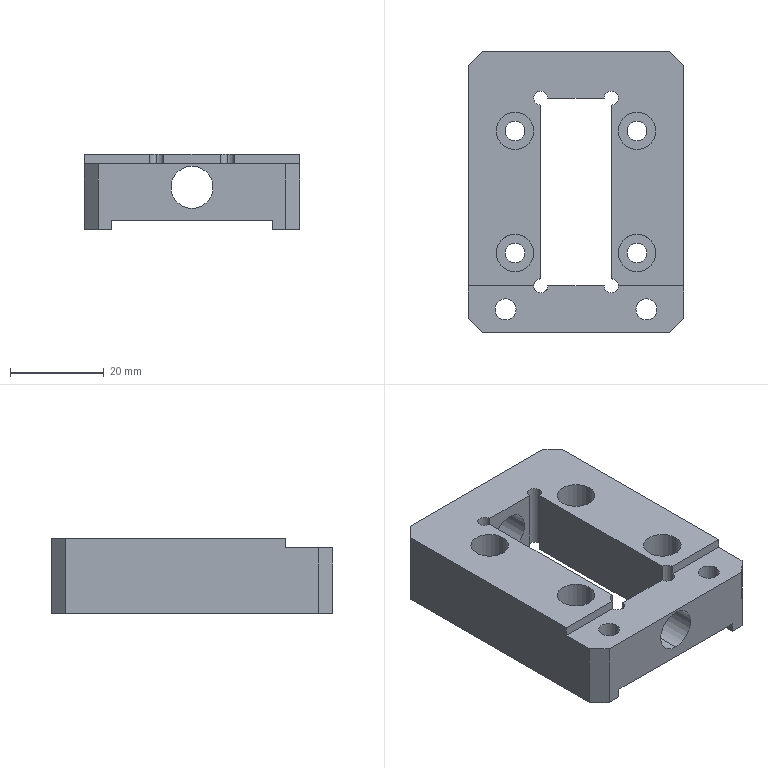Part | SolidWorks | features HoleWzd 5, ICE 4, Chamfer 3, Extrusion 1 | 1 solid | 63 faces | box 46 x 60 x 16 mm | volume 26364 mm3 | cylinder 34 | plane 29 | commonest cylinder face diameters 8 x12 4.2 x8 3 x6 4.5 x4 9 x4